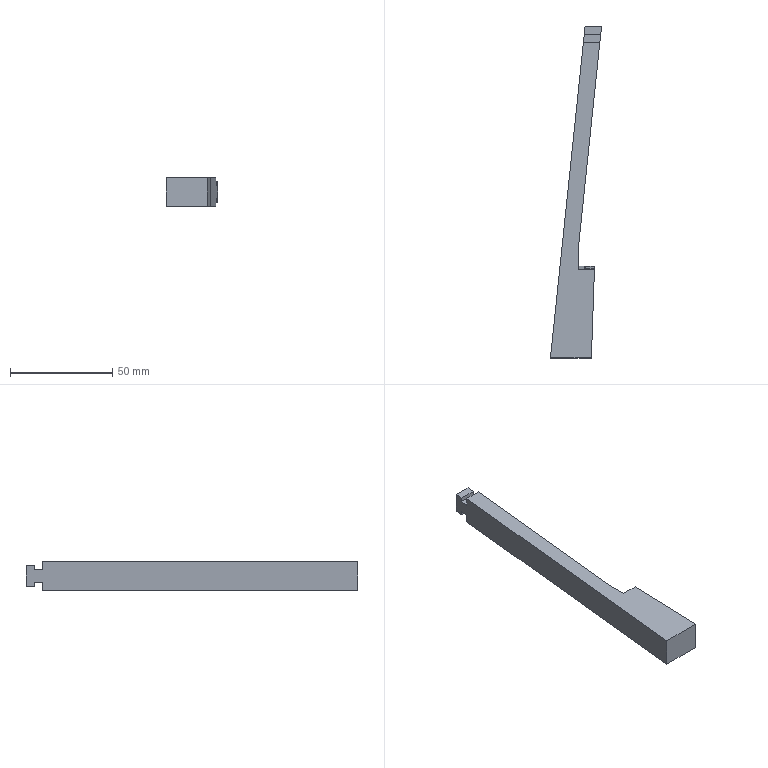Part | STEP file | 1 solid | 29 faces | box 24.981 x 162.36 x 14 mm | volume 24299 mm3 | plane 27 | cylinder 2 | commonest cylinder face diameters 1.005 x2